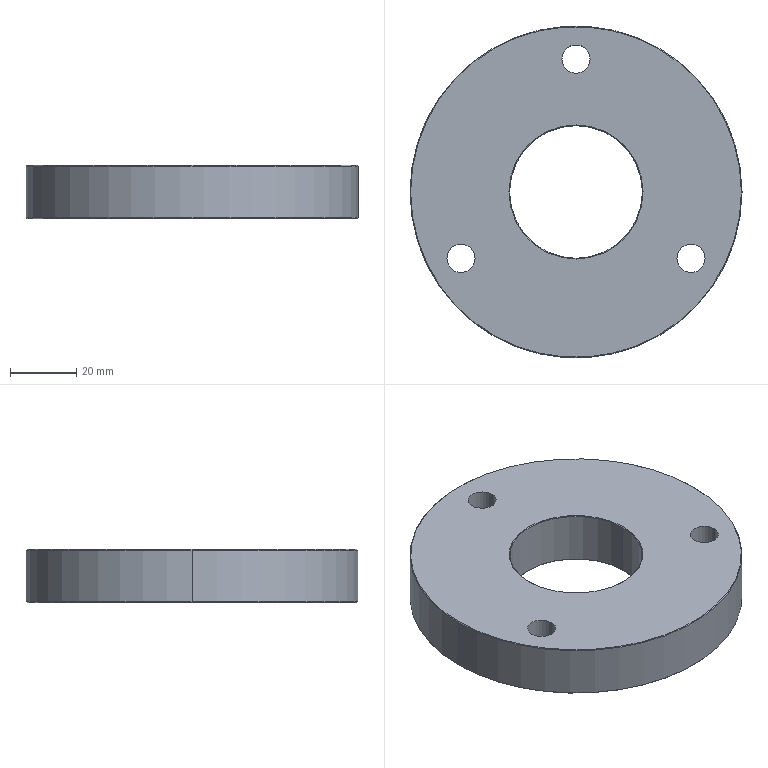Part | SolidWorks | features Chamfer 1, CirPattern 1, Extrusion 1, HoleWzd 1 | 1 solid | 20 faces | box 100 x 100 x 16 mm | volume 102816 mm3 | cylinder 10 | cone 8 | plane 2 | commonest cylinder face diameters 8.5 x6 40 x2 100 x2
STEP:
#1=CARTESIAN_POINT('',(49.8,0.,16.));
#2=VERTEX_POINT('',#1);
#3=CARTESIAN_POINT('',(-49.8,0.,16.));
#4=VERTEX_POINT('',#3);
#5=CARTESIAN_POINT('',(0.,0.,16.));
#6=DIRECTION('',(0.,0.,1.));
#7=DIRECTION('',(1.,0.,0.));
#8=AXIS2_PLACEMENT_3D('',#5,#6,#7);
#9=CIRCLE('',#8,49.8);
#10=EDGE_CURVE('',#2,#4,#9,.T.);
#11=ORIENTED_EDGE('',*,*,#10,.F.);
#12=CARTESIAN_POINT('',(50.,0.,15.8));
#13=VERTEX_POINT('',#12);
#14=CARTESIAN_POINT('',(49.8,0.,16.));
#15=DIRECTION('',(0.7071,0.,-0.7071));
#16=VECTOR('',#15,1000.);
#17=LINE('',#14,#16);
#18=EDGE_CURVE('',#2,#13,#17,.T.);
#19=ORIENTED_EDGE('',*,*,#18,.T.);
#20=CARTESIAN_POINT('',(-50.,0.,15.8));
#21=VERTEX_POINT('',#20);
#22=CARTESIAN_POINT('',(0.,0.,15.8));
#23=DIRECTION('',(0.,0.,-1.));
#24=DIRECTION('',(1.,0.,0.));
#25=AXIS2_PLACEMENT_3D('',#22,#23,#24);
#26=CIRCLE('',#25,50.);
#27=EDGE_CURVE('',#21,#13,#26,.T.);
#28=ORIENTED_EDGE('',*,*,#27,.F.);
#29=CARTESIAN_POINT('',(-49.8,0.,16.));
#30=DIRECTION('',(-0.7071,0.,-0.7071));
#31=VECTOR('',#30,1000.);
#32=LINE('',#29,#31);
#33=EDGE_CURVE('',#4,#21,#32,.T.);
#34=ORIENTED_EDGE('',*,*,#33,.F.);
#35=EDGE_LOOP('',(#11,#19,#28,#34));
#36=FACE_OUTER_BOUND('',#35,.T.);
#37=CARTESIAN_POINT('',(0.,0.,16.));
#38=DIRECTION('',(0.,0.,-1.));
#39=DIRECTION('',(-1.,0.,0.));
#40=AXIS2_PLACEMENT_3D('',#37,#38,#39);
#41=CONICAL_SURFACE('',#40,49.8,0.7854);
#42=ADVANCED_FACE('',(#36),#41,.T.);
#43=CARTESIAN_POINT('',(-49.8,0.,0.));
#44=VERTEX_POINT('',#43);
#45=CARTESIAN_POINT('',(49.8,0.,0.));
#46=VERTEX_POINT('',#45);
#47=CARTESIAN_POINT('',(0.,0.,0.));
#48=DIRECTION('',(0.,0.,-1.));
#49=DIRECTION('',(1.,0.,0.));
#50=AXIS2_PLACEMENT_3D('',#47,#48,#49);
#51=CIRCLE('',#50,49.8);
#52=EDGE_CURVE('',#44,#46,#51,.T.);
#53=ORIENTED_EDGE('',*,*,#52,.F.);
#54=CARTESIAN_POINT('',(-50.,0.,0.2));
#55=VERTEX_POINT('',#54);
#56=CARTESIAN_POINT('',(-50.,0.,0.2));
#57=DIRECTION('',(-0.7071,0.,0.7071));
#58=VECTOR('',#57,1000.);
#59=LINE('',#56,#58);
#60=EDGE_CURVE('',#44,#55,#59,.T.);
#61=ORIENTED_EDGE('',*,*,#60,.T.);
#62=CARTESIAN_POINT('',(50.,0.,0.2));
#63=VERTEX_POINT('',#62);
#64=CARTESIAN_POINT('',(0.,0.,0.2));
#65=DIRECTION('',(0.,0.,1.));
#66=DIRECTION('',(1.,0.,0.));
#67=AXIS2_PLACEMENT_3D('',#64,#65,#66);
#68=CIRCLE('',#67,50.);
#69=EDGE_CURVE('',#63,#55,#68,.T.);
#70=ORIENTED_EDGE('',*,*,#69,.F.);
#71=CARTESIAN_POINT('',(50.,0.,0.2));
#72=DIRECTION('',(0.7071,0.,0.7071));
#73=VECTOR('',#72,1000.);
#74=LINE('',#71,#73);
#75=EDGE_CURVE('',#46,#63,#74,.T.);
#76=ORIENTED_EDGE('',*,*,#75,.F.);
#77=EDGE_LOOP('',(#53,#61,#70,#76));
#78=FACE_OUTER_BOUND('',#77,.T.);
#79=CARTESIAN_POINT('',(0.,0.,0.2));
#80=DIRECTION('',(0.,0.,1.));
#81=DIRECTION('',(1.,0.,0.));
#82=AXIS2_PLACEMENT_3D('',#79,#80,#81);
#83=CONICAL_SURFACE('',#82,50.,0.7854);
#84=ADVANCED_FACE('',(#78),#83,.T.);
#85=CARTESIAN_POINT('',(20.,0.,0.2));
#86=VERTEX_POINT('',#85);
#87=CARTESIAN_POINT('',(-20.,0.,0.2));
#88=VERTEX_POINT('',#87);
#89=CARTESIAN_POINT('',(0.,0.,0.2));
#90=DIRECTION('',(0.,0.,-1.));
#91=DIRECTION('',(1.,0.,0.));
#92=AXIS2_PLACEMENT_3D('',#89,#90,#91);
#93=CIRCLE('',#92,20.);
#94=EDGE_CURVE('',#86,#88,#93,.T.);
#95=ORIENTED_EDGE('',*,*,#94,.F.);
#96=CARTESIAN_POINT('',(20.2,0.,0.));
#97=VERTEX_POINT('',#96);
#98=CARTESIAN_POINT('',(20.2,0.,0.));
#99=DIRECTION('',(0.7071,0.,-0.7071));
#100=VECTOR('',#99,1000.);
#101=LINE('',#98,#100);
#102=EDGE_CURVE('',#86,#97,#101,.T.);
#103=ORIENTED_EDGE('',*,*,#102,.T.);
#104=CARTESIAN_POINT('',(-20.2,0.,0.));
#105=VERTEX_POINT('',#104);
#106=CARTESIAN_POINT('',(0.,0.,0.));
#107=DIRECTION('',(0.,0.,1.));
#108=DIRECTION('',(1.,0.,0.));
#109=AXIS2_PLACEMENT_3D('',#106,#107,#108);
#110=CIRCLE('',#109,20.2);
#111=EDGE_CURVE('',#105,#97,#110,.T.);
#112=ORIENTED_EDGE('',*,*,#111,.F.);
#113=CARTESIAN_POINT('',(-20.2,0.,0.));
#114=DIRECTION('',(-0.7071,0.,-0.7071));
#115=VECTOR('',#114,1000.);
#116=LINE('',#113,#115);
#117=EDGE_CURVE('',#88,#105,#116,.T.);
#118=ORIENTED_EDGE('',*,*,#117,.F.);
#119=EDGE_LOOP('',(#95,#103,#112,#118));
#120=FACE_OUTER_BOUND('',#119,.T.);
#121=CARTESIAN_POINT('',(0.,0.,0.));
#122=DIRECTION('',(0.,0.,-1.));
#123=DIRECTION('',(-1.,0.,0.));
#124=AXIS2_PLACEMENT_3D('',#121,#122,#123);
#125=CONICAL_SURFACE('',#124,20.2,0.7854);
#126=ADVANCED_FACE('',(#120),#125,.F.);
#127=CARTESIAN_POINT('',(-20.,0.,15.8));
#128=VERTEX_POINT('',#127);
#129=CARTESIAN_POINT('',(20.,0.,15.8));
#130=VERTEX_POINT('',#129);
#131=CARTESIAN_POINT('',(0.,0.,15.8));
#132=DIRECTION('',(0.,0.,1.));
#133=DIRECTION('',(1.,0.,0.));
#134=AXIS2_PLACEMENT_3D('',#131,#132,#133);
#135=CIRCLE('',#134,20.);
#136=EDGE_CURVE('',#128,#130,#135,.T.);
#137=ORIENTED_EDGE('',*,*,#136,.F.);
#138=CARTESIAN_POINT('',(-20.2,0.,16.));
#139=VERTEX_POINT('',#138);
#140=CARTESIAN_POINT('',(-20.,0.,15.8));
#141=DIRECTION('',(-0.7071,0.,0.7071));
#142=VECTOR('',#141,1000.);
#143=LINE('',#140,#142);
#144=EDGE_CURVE('',#128,#139,#143,.T.);
#145=ORIENTED_EDGE('',*,*,#144,.T.);
#146=CARTESIAN_POINT('',(20.2,0.,16.));
#147=VERTEX_POINT('',#146);
#148=CARTESIAN_POINT('',(0.,0.,16.));
#149=DIRECTION('',(0.,0.,-1.));
#150=DIRECTION('',(1.,0.,0.));
#151=AXIS2_PLACEMENT_3D('',#148,#149,#150);
#152=CIRCLE('',#151,20.2);
#153=EDGE_CURVE('',#147,#139,#152,.T.);
#154=ORIENTED_EDGE('',*,*,#153,.F.);
#155=CARTESIAN_POINT('',(20.,0.,15.8));
#156=DIRECTION('',(0.7071,0.,0.7071));
#157=VECTOR('',#156,1000.);
#158=LINE('',#155,#157);
#159=EDGE_CURVE('',#130,#147,#158,.T.);
#160=ORIENTED_EDGE('',*,*,#159,.F.);
#161=EDGE_LOOP('',(#137,#145,#154,#160));
#162=FACE_OUTER_BOUND('',#161,.T.);
#163=CARTESIAN_POINT('',(0.,0.,15.8));
#164=DIRECTION('',(0.,0.,1.));
#165=DIRECTION('',(1.,0.,0.));
#166=AXIS2_PLACEMENT_3D('',#163,#164,#165);
#167=CONICAL_SURFACE('',#166,20.,0.7854);
#168=ADVANCED_FACE('',(#162),#167,.F.);
#169=CARTESIAN_POINT('',(-38.891,-20.,0.));
#170=VERTEX_POINT('',#169);
#171=CARTESIAN_POINT('',(-30.391,-20.,0.));
#172=VERTEX_POINT('',#171);
#173=CARTESIAN_POINT('',(-34.641,-20.,0.));
#174=DIRECTION('',(0.,0.,1.));
#175=DIRECTION('',(1.,0.,0.));
#176=AXIS2_PLACEMENT_3D('',#173,#174,#175);
#177=CIRCLE('',#176,4.25);
#178=EDGE_CURVE('',#170,#172,#177,.T.);
#179=ORIENTED_EDGE('',*,*,#178,.F.);
#180=CARTESIAN_POINT('',(-38.891,-20.,16.));
#181=VERTEX_POINT('',#180);
#182=CARTESIAN_POINT('',(-38.891,-20.,16.));
#183=DIRECTION('',(0.,0.,1.));
#184=VECTOR('',#183,1000.);
#185=LINE('',#182,#184);
#186=EDGE_CURVE('',#170,#181,#185,.T.);
#187=ORIENTED_EDGE('',*,*,#186,.T.);
#188=CARTESIAN_POINT('',(-30.391,-20.,16.));
#189=VERTEX_POINT('',#188);
#190=CARTESIAN_POINT('',(-34.641,-20.,16.));
#191=DIRECTION('',(0.,0.,1.));
#192=DIRECTION('',(1.,0.,0.));
#193=AXIS2_PLACEMENT_3D('',#190,#191,#192);
#194=CIRCLE('',#193,4.25);
#195=EDGE_CURVE('',#181,#189,#194,.T.);
#196=ORIENTED_EDGE('',*,*,#195,.T.);
#197=CARTESIAN_POINT('',(-30.391,-20.,16.));
#198=DIRECTION('',(0.,0.,1.));
#199=VECTOR('',#198,1000.);
#200=LINE('',#197,#199);
#201=EDGE_CURVE('',#172,#189,#200,.T.);
#202=ORIENTED_EDGE('',*,*,#201,.F.);
#203=EDGE_LOOP('',(#179,#187,#196,#202));
#204=FACE_OUTER_BOUND('',#203,.T.);
#205=CARTESIAN_POINT('',(-34.641,-20.,16.));
#206=DIRECTION('',(0.,0.,1.));
#207=DIRECTION('',(1.,0.,0.));
#208=AXIS2_PLACEMENT_3D('',#205,#206,#207);
#209=CYLINDRICAL_SURFACE('',#208,4.25);
#210=ADVANCED_FACE('',(#204),#209,.F.);
#211=CARTESIAN_POINT('',(30.391,-20.,0.));
#212=VERTEX_POINT('',#211);
#213=CARTESIAN_POINT('',(38.891,-20.,0.));
#214=VERTEX_POINT('',#213);
#215=CARTESIAN_POINT('',(34.641,-20.,0.));
#216=DIRECTION('',(0.,0.,1.));
#217=DIRECTION('',(1.,0.,0.));
#218=AXIS2_PLACEMENT_3D('',#215,#216,#217);
#219=CIRCLE('',#218,4.25);
#220=EDGE_CURVE('',#212,#214,#219,.T.);
#221=ORIENTED_EDGE('',*,*,#220,.F.);
#222=CARTESIAN_POINT('',(30.391,-20.,16.));
#223=VERTEX_POINT('',#222);
#224=CARTESIAN_POINT('',(30.391,-20.,16.));
#225=DIRECTION('',(0.,0.,1.));
#226=VECTOR('',#225,1000.);
#227=LINE('',#224,#226);
#228=EDGE_CURVE('',#212,#223,#227,.T.);
#229=ORIENTED_EDGE('',*,*,#228,.T.);
#230=CARTESIAN_POINT('',(38.891,-20.,16.));
#231=VERTEX_POINT('',#230);
#232=CARTESIAN_POINT('',(34.641,-20.,16.));
#233=DIRECTION('',(0.,0.,1.));
#234=DIRECTION('',(1.,0.,0.));
#235=AXIS2_PLACEMENT_3D('',#232,#233,#234);
#236=CIRCLE('',#235,4.25);
#237=EDGE_CURVE('',#223,#231,#236,.T.);
#238=ORIENTED_EDGE('',*,*,#237,.T.);
#239=CARTESIAN_POINT('',(38.891,-20.,16.));
#240=DIRECTION('',(0.,0.,1.));
#241=VECTOR('',#240,1000.);
#242=LINE('',#239,#241);
#243=EDGE_CURVE('',#214,#231,#242,.T.);
#244=ORIENTED_EDGE('',*,*,#243,.F.);
#245=EDGE_LOOP('',(#221,#229,#238,#244));
#246=FACE_OUTER_BOUND('',#245,.T.);
#247=CARTESIAN_POINT('',(34.641,-20.,16.));
#248=DIRECTION('',(0.,0.,1.));
#249=DIRECTION('',(1.,0.,0.));
#250=AXIS2_PLACEMENT_3D('',#247,#248,#249);
#251=CYLINDRICAL_SURFACE('',#250,4.25);
#252=ADVANCED_FACE('',(#246),#251,.F.);
#253=CARTESIAN_POINT('',(-4.25,40.,0.));
#254=VERTEX_POINT('',#253);
#255=CARTESIAN_POINT('',(4.25,40.,0.));
#256=VERTEX_POINT('',#255);
#257=CARTESIAN_POINT('',(0.,40.,0.));
#258=DIRECTION('',(0.,0.,1.));
#259=DIRECTION('',(1.,0.,0.));
#260=AXIS2_PLACEMENT_3D('',#257,#258,#259);
#261=CIRCLE('',#260,4.25);
#262=EDGE_CURVE('',#254,#256,#261,.T.);
#263=ORIENTED_EDGE('',*,*,#262,.F.);
#264=CARTESIAN_POINT('',(-4.25,40.,16.));
#265=VERTEX_POINT('',#264);
#266=CARTESIAN_POINT('',(-4.25,40.,16.));
#267=DIRECTION('',(0.,0.,1.));
#268=VECTOR('',#267,1000.);
#269=LINE('',#266,#268);
#270=EDGE_CURVE('',#254,#265,#269,.T.);
#271=ORIENTED_EDGE('',*,*,#270,.T.);
#272=CARTESIAN_POINT('',(4.25,40.,16.));
#273=VERTEX_POINT('',#272);
#274=CARTESIAN_POINT('',(0.,40.,16.));
#275=DIRECTION('',(0.,0.,1.));
#276=DIRECTION('',(1.,0.,0.));
#277=AXIS2_PLACEMENT_3D('',#274,#275,#276);
#278=CIRCLE('',#277,4.25);
#279=EDGE_CURVE('',#265,#273,#278,.T.);
#280=ORIENTED_EDGE('',*,*,#279,.T.);
#281=CARTESIAN_POINT('',(4.25,40.,16.));
#282=DIRECTION('',(0.,0.,1.));
#283=VECTOR('',#282,1000.);
#284=LINE('',#281,#283);
#285=EDGE_CURVE('',#256,#273,#284,.T.);
#286=ORIENTED_EDGE('',*,*,#285,.F.);
#287=EDGE_LOOP('',(#263,#271,#280,#286));
#288=FACE_OUTER_BOUND('',#287,.T.);
#289=CARTESIAN_POINT('',(0.,40.,16.));
#290=DIRECTION('',(0.,0.,1.));
#291=DIRECTION('',(1.,0.,0.));
#292=AXIS2_PLACEMENT_3D('',#289,#290,#291);
#293=CYLINDRICAL_SURFACE('',#292,4.25);
#294=ADVANCED_FACE('',(#288),#293,.F.);
#295=ORIENTED_EDGE('',*,*,#136,.T.);
#296=CARTESIAN_POINT('',(20.,0.,16.));
#297=DIRECTION('',(0.,0.,-1.));
#298=VECTOR('',#297,1000.);
#299=LINE('',#296,#298);
#300=EDGE_CURVE('',#130,#86,#299,.T.);
#301=ORIENTED_EDGE('',*,*,#300,.T.);
#302=ORIENTED_EDGE('',*,*,#94,.T.);
#303=CARTESIAN_POINT('',(-20.,0.,16.));
#304=DIRECTION('',(0.,0.,-1.));
#305=VECTOR('',#304,1000.);
#306=LINE('',#303,#305);
#307=EDGE_CURVE('',#128,#88,#306,.T.);
#308=ORIENTED_EDGE('',*,*,#307,.F.);
#309=EDGE_LOOP('',(#295,#301,#302,#308));
#310=FACE_OUTER_BOUND('',#309,.T.);
#311=CARTESIAN_POINT('',(0.,0.,16.));
#312=DIRECTION('',(0.,0.,-1.));
#313=DIRECTION('',(-1.,0.,0.));
#314=AXIS2_PLACEMENT_3D('',#311,#312,#313);
#315=CYLINDRICAL_SURFACE('',#314,20.);
#316=ADVANCED_FACE('',(#310),#315,.F.);
#317=ORIENTED_EDGE('',*,*,#27,.T.);
#318=CARTESIAN_POINT('',(50.,0.,16.));
#319=DIRECTION('',(0.,0.,-1.));
#320=VECTOR('',#319,1000.);
#321=LINE('',#318,#320);
#322=EDGE_CURVE('',#13,#63,#321,.T.);
#323=ORIENTED_EDGE('',*,*,#322,.T.);
#324=ORIENTED_EDGE('',*,*,#69,.T.);
#325=CARTESIAN_POINT('',(-50.,0.,16.));
#326=DIRECTION('',(0.,0.,-1.));
#327=VECTOR('',#326,1000.);
#328=LINE('',#325,#327);
#329=EDGE_CURVE('',#21,#55,#328,.T.);
#330=ORIENTED_EDGE('',*,*,#329,.F.);
#331=EDGE_LOOP('',(#317,#323,#324,#330));
#332=FACE_OUTER_BOUND('',#331,.T.);
#333=CARTESIAN_POINT('',(0.,0.,16.));
#334=DIRECTION('',(0.,0.,-1.));
#335=DIRECTION('',(-1.,0.,0.));
#336=AXIS2_PLACEMENT_3D('',#333,#334,#335);
#337=CYLINDRICAL_SURFACE('',#336,50.);
#338=ADVANCED_FACE('',(#332),#337,.T.);
#339=ORIENTED_EDGE('',*,*,#153,.T.);
#340=CARTESIAN_POINT('',(0.,0.,16.));
#341=DIRECTION('',(0.,0.,-1.));
#342=DIRECTION('',(1.,0.,0.));
#343=AXIS2_PLACEMENT_3D('',#340,#341,#342);
#344=CIRCLE('',#343,20.2);
#345=EDGE_CURVE('',#139,#147,#344,.T.);
#346=ORIENTED_EDGE('',*,*,#345,.T.);
#347=EDGE_LOOP('',(#339,#346));
#348=FACE_BOUND('',#347,.T.);
#349=CARTESIAN_POINT('',(0.,0.,16.));
#350=DIRECTION('',(0.,0.,1.));
#351=DIRECTION('',(1.,0.,0.));
#352=AXIS2_PLACEMENT_3D('',#349,#350,#351);
#353=CIRCLE('',#352,49.8);
#354=EDGE_CURVE('',#4,#2,#353,.T.);
#355=ORIENTED_EDGE('',*,*,#354,.T.);
#356=ORIENTED_EDGE('',*,*,#10,.T.);
#357=EDGE_LOOP('',(#355,#356));
#358=FACE_OUTER_BOUND('',#357,.T.);
#359=CARTESIAN_POINT('',(-34.641,-20.,16.));
#360=DIRECTION('',(0.,0.,1.));
#361=DIRECTION('',(1.,0.,0.));
#362=AXIS2_PLACEMENT_3D('',#359,#360,#361);
#363=CIRCLE('',#362,4.25);
#364=EDGE_CURVE('',#189,#181,#363,.T.);
#365=ORIENTED_EDGE('',*,*,#364,.F.);
#366=ORIENTED_EDGE('',*,*,#195,.F.);
#367=EDGE_LOOP('',(#365,#366));
#368=FACE_BOUND('',#367,.T.);
#369=CARTESIAN_POINT('',(34.641,-20.,16.));
#370=DIRECTION('',(0.,0.,1.));
#371=DIRECTION('',(1.,0.,0.));
#372=AXIS2_PLACEMENT_3D('',#369,#370,#371);
#373=CIRCLE('',#372,4.25);
#374=EDGE_CURVE('',#231,#223,#373,.T.);
#375=ORIENTED_EDGE('',*,*,#374,.F.);
#376=ORIENTED_EDGE('',*,*,#237,.F.);
#377=EDGE_LOOP('',(#375,#376));
#378=FACE_BOUND('',#377,.T.);
#379=CARTESIAN_POINT('',(0.,40.,16.));
#380=DIRECTION('',(0.,0.,1.));
#381=DIRECTION('',(1.,0.,0.));
#382=AXIS2_PLACEMENT_3D('',#379,#380,#381);
#383=CIRCLE('',#382,4.25);
#384=EDGE_CURVE('',#273,#265,#383,.T.);
#385=ORIENTED_EDGE('',*,*,#384,.F.);
#386=ORIENTED_EDGE('',*,*,#279,.F.);
#387=EDGE_LOOP('',(#385,#386));
#388=FACE_BOUND('',#387,.T.);
#389=CARTESIAN_POINT('',(0.,0.,16.));
#390=DIRECTION('',(0.,0.,1.));
#391=DIRECTION('',(1.,0.,0.));
#392=AXIS2_PLACEMENT_3D('',#389,#390,#391);
#393=PLANE('',#392);
#394=ADVANCED_FACE('',(#348,#358,#368,#378,#388),#393,.T.);
#395=ORIENTED_EDGE('',*,*,#111,.T.);
#396=CARTESIAN_POINT('',(0.,0.,0.));
#397=DIRECTION('',(0.,0.,1.));
#398=DIRECTION('',(1.,0.,0.));
#399=AXIS2_PLACEMENT_3D('',#396,#397,#398);
#400=CIRCLE('',#399,20.2);
#401=EDGE_CURVE('',#97,#105,#400,.T.);
#402=ORIENTED_EDGE('',*,*,#401,.T.);
#403=EDGE_LOOP('',(#395,#402));
#404=FACE_BOUND('',#403,.T.);
#405=CARTESIAN_POINT('',(0.,0.,0.));
#406=DIRECTION('',(0.,0.,-1.));
#407=DIRECTION('',(1.,0.,0.));
#408=AXIS2_PLACEMENT_3D('',#405,#406,#407);
#409=CIRCLE('',#408,49.8);
#410=EDGE_CURVE('',#46,#44,#409,.T.);
#411=ORIENTED_EDGE('',*,*,#410,.T.);
#412=ORIENTED_EDGE('',*,*,#52,.T.);
#413=EDGE_LOOP('',(#411,#412));
#414=FACE_OUTER_BOUND('',#413,.T.);
#415=CARTESIAN_POINT('',(-34.641,-20.,0.));
#416=DIRECTION('',(0.,0.,1.));
#417=DIRECTION('',(1.,0.,0.));
#418=AXIS2_PLACEMENT_3D('',#415,#416,#417);
#419=CIRCLE('',#418,4.25);
#420=EDGE_CURVE('',#172,#170,#419,.T.);
#421=ORIENTED_EDGE('',*,*,#420,.T.);
#422=ORIENTED_EDGE('',*,*,#178,.T.);
#423=EDGE_LOOP('',(#421,#422));
#424=FACE_BOUND('',#423,.T.);
#425=CARTESIAN_POINT('',(34.641,-20.,0.));
#426=DIRECTION('',(0.,0.,1.));
#427=DIRECTION('',(1.,0.,0.));
#428=AXIS2_PLACEMENT_3D('',#425,#426,#427);
#429=CIRCLE('',#428,4.25);
#430=EDGE_CURVE('',#214,#212,#429,.T.);
#431=ORIENTED_EDGE('',*,*,#430,.T.);
#432=ORIENTED_EDGE('',*,*,#220,.T.);
#433=EDGE_LOOP('',(#431,#432));
#434=FACE_BOUND('',#433,.T.);
#435=CARTESIAN_POINT('',(0.,40.,0.));
#436=DIRECTION('',(0.,0.,1.));
#437=DIRECTION('',(1.,0.,0.));
#438=AXIS2_PLACEMENT_3D('',#435,#436,#437);
#439=CIRCLE('',#438,4.25);
#440=EDGE_CURVE('',#256,#254,#439,.T.);
#441=ORIENTED_EDGE('',*,*,#440,.T.);
#442=ORIENTED_EDGE('',*,*,#262,.T.);
#443=EDGE_LOOP('',(#441,#442));
#444=FACE_BOUND('',#443,.T.);
#445=CARTESIAN_POINT('',(0.,0.,0.));
#446=DIRECTION('',(0.,0.,1.));
#447=DIRECTION('',(1.,0.,0.));
#448=AXIS2_PLACEMENT_3D('',#445,#446,#447);
#449=PLANE('',#448);
#450=ADVANCED_FACE('',(#404,#414,#424,#434,#444),#449,.F.);
#451=ORIENTED_EDGE('',*,*,#322,.F.);
#452=CARTESIAN_POINT('',(0.,0.,15.8));
#453=DIRECTION('',(0.,0.,-1.));
#454=DIRECTION('',(1.,0.,0.));
#455=AXIS2_PLACEMENT_3D('',#452,#453,#454);
#456=CIRCLE('',#455,50.);
#457=EDGE_CURVE('',#13,#21,#456,.T.);
#458=ORIENTED_EDGE('',*,*,#457,.T.);
#459=ORIENTED_EDGE('',*,*,#329,.T.);
#460=CARTESIAN_POINT('',(0.,0.,0.2));
#461=DIRECTION('',(0.,0.,1.));
#462=DIRECTION('',(1.,0.,0.));
#463=AXIS2_PLACEMENT_3D('',#460,#461,#462);
#464=CIRCLE('',#463,50.);
#465=EDGE_CURVE('',#55,#63,#464,.T.);
#466=ORIENTED_EDGE('',*,*,#465,.T.);
#467=EDGE_LOOP('',(#451,#458,#459,#466));
#468=FACE_OUTER_BOUND('',#467,.T.);
#469=CARTESIAN_POINT('',(0.,0.,16.));
#470=DIRECTION('',(0.,0.,-1.));
#471=DIRECTION('',(-1.,0.,0.));
#472=AXIS2_PLACEMENT_3D('',#469,#470,#471);
#473=CYLINDRICAL_SURFACE('',#472,50.);
#474=ADVANCED_FACE('',(#468),#473,.T.);
#475=ORIENTED_EDGE('',*,*,#300,.F.);
#476=CARTESIAN_POINT('',(0.,0.,15.8));
#477=DIRECTION('',(0.,0.,1.));
#478=DIRECTION('',(1.,0.,0.));
#479=AXIS2_PLACEMENT_3D('',#476,#477,#478);
#480=CIRCLE('',#479,20.);
#481=EDGE_CURVE('',#130,#128,#480,.T.);
#482=ORIENTED_EDGE('',*,*,#481,.T.);
#483=ORIENTED_EDGE('',*,*,#307,.T.);
#484=CARTESIAN_POINT('',(0.,0.,0.2));
#485=DIRECTION('',(0.,0.,-1.));
#486=DIRECTION('',(1.,0.,0.));
#487=AXIS2_PLACEMENT_3D('',#484,#485,#486);
#488=CIRCLE('',#487,20.);
#489=EDGE_CURVE('',#88,#86,#488,.T.);
#490=ORIENTED_EDGE('',*,*,#489,.T.);
#491=EDGE_LOOP('',(#475,#482,#483,#490));
#492=FACE_OUTER_BOUND('',#491,.T.);
#493=CARTESIAN_POINT('',(0.,0.,16.));
#494=DIRECTION('',(0.,0.,-1.));
#495=DIRECTION('',(-1.,0.,0.));
#496=AXIS2_PLACEMENT_3D('',#493,#494,#495);
#497=CYLINDRICAL_SURFACE('',#496,20.);
#498=ADVANCED_FACE('',(#492),#497,.F.);
#499=ORIENTED_EDGE('',*,*,#270,.F.);
#500=ORIENTED_EDGE('',*,*,#440,.F.);
#501=ORIENTED_EDGE('',*,*,#285,.T.);
#502=ORIENTED_EDGE('',*,*,#384,.T.);
#503=EDGE_LOOP('',(#499,#500,#501,#502));
#504=FACE_OUTER_BOUND('',#503,.T.);
#505=CARTESIAN_POINT('',(0.,40.,16.));
#506=DIRECTION('',(0.,0.,1.));
#507=DIRECTION('',(1.,0.,0.));
#508=AXIS2_PLACEMENT_3D('',#505,#506,#507);
#509=CYLINDRICAL_SURFACE('',#508,4.25);
#510=ADVANCED_FACE('',(#504),#509,.F.);
#511=ORIENTED_EDGE('',*,*,#228,.F.);
#512=ORIENTED_EDGE('',*,*,#430,.F.);
#513=ORIENTED_EDGE('',*,*,#243,.T.);
#514=ORIENTED_EDGE('',*,*,#374,.T.);
#515=EDGE_LOOP('',(#511,#512,#513,#514));
#516=FACE_OUTER_BOUND('',#515,.T.);
#517=CARTESIAN_POINT('',(34.641,-20.,16.));
#518=DIRECTION('',(0.,0.,1.));
#519=DIRECTION('',(1.,0.,0.));
#520=AXIS2_PLACEMENT_3D('',#517,#518,#519);
#521=CYLINDRICAL_SURFACE('',#520,4.25);
#522=ADVANCED_FACE('',(#516),#521,.F.);
#523=ORIENTED_EDGE('',*,*,#186,.F.);
#524=ORIENTED_EDGE('',*,*,#420,.F.);
#525=ORIENTED_EDGE('',*,*,#201,.T.);
#526=ORIENTED_EDGE('',*,*,#364,.T.);
#527=EDGE_LOOP('',(#523,#524,#525,#526));
#528=FACE_OUTER_BOUND('',#527,.T.);
#529=CARTESIAN_POINT('',(-34.641,-20.,16.));
#530=DIRECTION('',(0.,0.,1.));
#531=DIRECTION('',(1.,0.,0.));
#532=AXIS2_PLACEMENT_3D('',#529,#530,#531);
#533=CYLINDRICAL_SURFACE('',#532,4.25);
#534=ADVANCED_FACE('',(#528),#533,.F.);
#535=ORIENTED_EDGE('',*,*,#144,.F.);
#536=ORIENTED_EDGE('',*,*,#481,.F.);
#537=ORIENTED_EDGE('',*,*,#159,.T.);
#538=ORIENTED_EDGE('',*,*,#345,.F.);
#539=EDGE_LOOP('',(#535,#536,#537,#538));
#540=FACE_OUTER_BOUND('',#539,.T.);
#541=CARTESIAN_POINT('',(0.,0.,15.8));
#542=DIRECTION('',(0.,0.,1.));
#543=DIRECTION('',(1.,0.,0.));
#544=AXIS2_PLACEMENT_3D('',#541,#542,#543);
#545=CONICAL_SURFACE('',#544,20.,0.7854);
#546=ADVANCED_FACE('',(#540),#545,.F.);
#547=ORIENTED_EDGE('',*,*,#102,.F.);
#548=ORIENTED_EDGE('',*,*,#489,.F.);
#549=ORIENTED_EDGE('',*,*,#117,.T.);
#550=ORIENTED_EDGE('',*,*,#401,.F.);
#551=EDGE_LOOP('',(#547,#548,#549,#550));
#552=FACE_OUTER_BOUND('',#551,.T.);
#553=CARTESIAN_POINT('',(0.,0.,0.));
#554=DIRECTION('',(0.,0.,-1.));
#555=DIRECTION('',(-1.,0.,0.));
#556=AXIS2_PLACEMENT_3D('',#553,#554,#555);
#557=CONICAL_SURFACE('',#556,20.2,0.7854);
#558=ADVANCED_FACE('',(#552),#557,.F.);
#559=ORIENTED_EDGE('',*,*,#60,.F.);
#560=ORIENTED_EDGE('',*,*,#410,.F.);
#561=ORIENTED_EDGE('',*,*,#75,.T.);
#562=ORIENTED_EDGE('',*,*,#465,.F.);
#563=EDGE_LOOP('',(#559,#560,#561,#562));
#564=FACE_OUTER_BOUND('',#563,.T.);
#565=CARTESIAN_POINT('',(0.,0.,0.2));
#566=DIRECTION('',(0.,0.,1.));
#567=DIRECTION('',(1.,0.,0.));
#568=AXIS2_PLACEMENT_3D('',#565,#566,#567);
#569=CONICAL_SURFACE('',#568,50.,0.7854);
#570=ADVANCED_FACE('',(#564),#569,.T.);
#571=ORIENTED_EDGE('',*,*,#18,.F.);
#572=ORIENTED_EDGE('',*,*,#354,.F.);
#573=ORIENTED_EDGE('',*,*,#33,.T.);
#574=ORIENTED_EDGE('',*,*,#457,.F.);
#575=EDGE_LOOP('',(#571,#572,#573,#574));
#576=FACE_OUTER_BOUND('',#575,.T.);
#577=CARTESIAN_POINT('',(0.,0.,16.));
#578=DIRECTION('',(0.,0.,-1.));
#579=DIRECTION('',(-1.,0.,0.));
#580=AXIS2_PLACEMENT_3D('',#577,#578,#579);
#581=CONICAL_SURFACE('',#580,49.8,0.7854);
#582=ADVANCED_FACE('',(#576),#581,.T.);
#583=CLOSED_SHELL('',(#42,#84,#126,#168,#210,#252,#294,#316,#338,#394,#450,#474,#498,#510,#522,#534,#546,#558,#570,#582));
#584=MANIFOLD_SOLID_BREP('',#583);
#585=CARTESIAN_POINT('',(0.,0.,0.));
#586=DIRECTION('',(0.,0.,1.));
#587=DIRECTION('',(1.,0.,0.));
#588=AXIS2_PLACEMENT_3D('',#585,#586,#587);
#589=(LENGTH_UNIT()NAMED_UNIT(*)SI_UNIT(.MILLI.,.METRE.));
#590=UNCERTAINTY_MEASURE_WITH_UNIT(LENGTH_MEASURE(0.00001),#589,'','');
#591=(NAMED_UNIT(*)PLANE_ANGLE_UNIT()SI_UNIT($,.RADIAN.));
#592=(NAMED_UNIT(*)SI_UNIT($,.STERADIAN.)SOLID_ANGLE_UNIT());
#593=(GEOMETRIC_REPRESENTATION_CONTEXT(3)GLOBAL_UNCERTAINTY_ASSIGNED_CONTEXT((#590))GLOBAL_UNIT_ASSIGNED_CONTEXT((#589,#591,#592))REPRESENTATION_CONTEXT('',''));
#594=ADVANCED_BREP_SHAPE_REPRESENTATION('',(#584,#588),#593);